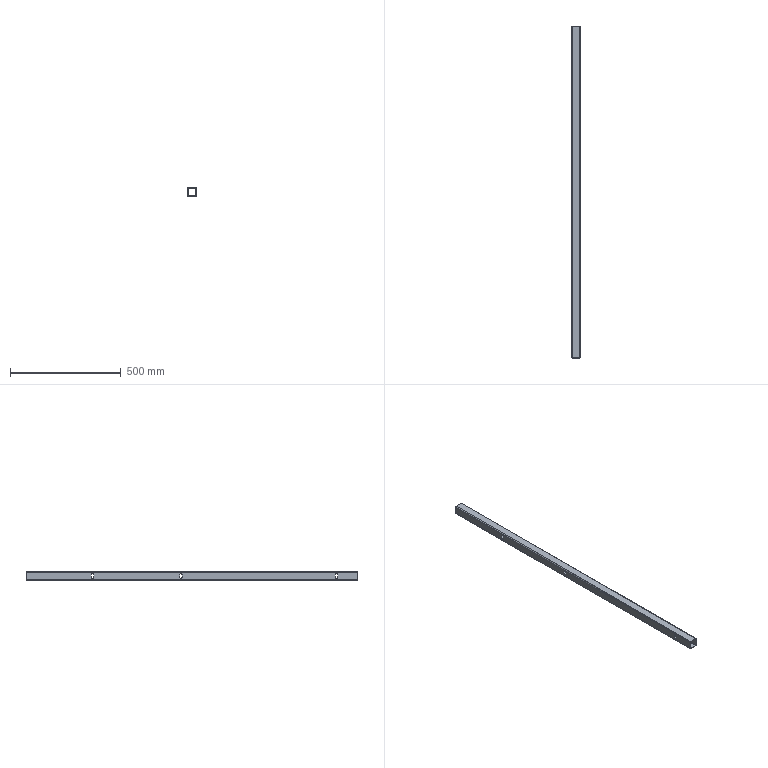Part | STEP file | E3-粉仓护栏10-1立柱主体_Default<As Machined> | 1 solid | 48 faces | box 40 x 1500 x 40 mm | volume 437751 mm3 | cylinder 26 | plane 22 | commonest cylinder face diameters 12 x18 4 x4 8 x4